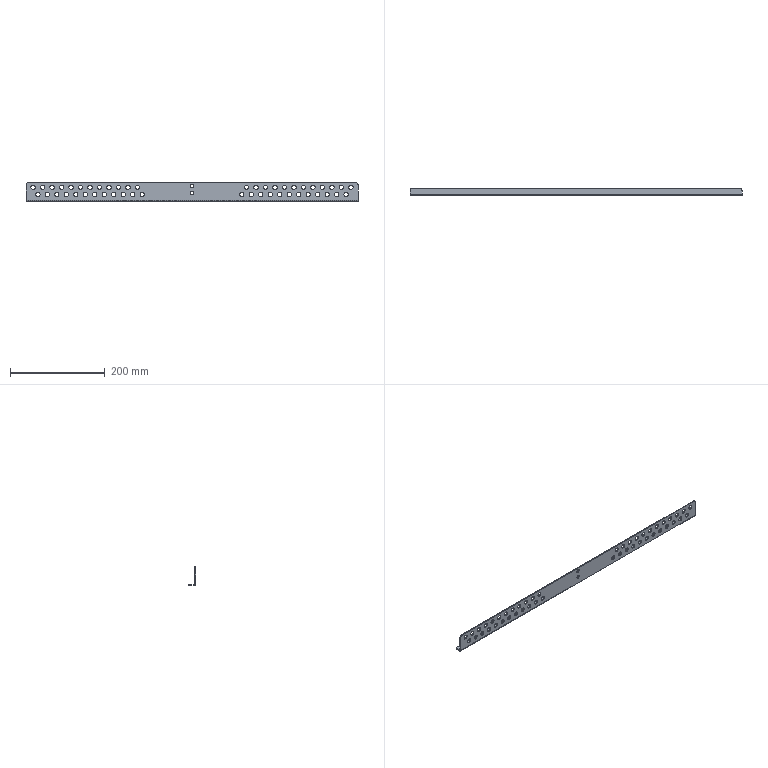Part | SolidWorks | features ICE 3, LPattern 2, MirrorPattern 2, EdgeFlange 1, Fillet 1, FlatPattern 1, SMBaseFlange 1, SheetMetal 1 | 1 solid | 118 faces | box 700 x 15 x 40 mm | volume 66578 mm3 | cylinder 106 | plane 12 | commonest cylinder face diameters 9.2 x96 7 x4 10 x4 1.473 x1 5.473 x1